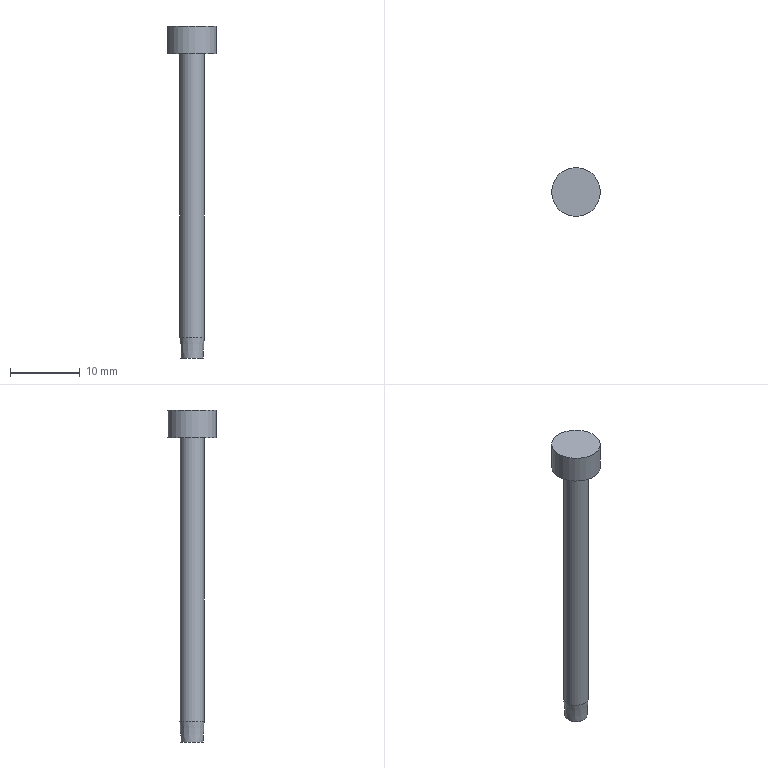Part | NX | features solid 2 | 1 solid | 6 faces | box 7 x 7 x 47.69 mm | volume 571.768 mm3 | plane 3 | cylinder 2 | cone 1 | commonest cylinder face diameters 3.5 x1 7 x1
STEP:
#1=CARTESIAN_POINT('',(-31.9,0.,66.5));
#2=VERTEX_POINT('',#1);
#3=CARTESIAN_POINT('',(-30.15,0.,66.5));
#4=DIRECTION('',(0.,0.,-1.));
#5=DIRECTION('',(-1.,0.,0.));
#6=AXIS2_PLACEMENT_3D('',#3,#4,#5);
#7=CIRCLE('',#6,1.75);
#8=EDGE_CURVE('',#2,#2,#7,.T.);
#9=ORIENTED_EDGE('',*,*,#8,.T.);
#10=EDGE_LOOP('',(#9));
#11=FACE_BOUND('',#10,.T.);
#12=CARTESIAN_POINT('',(-28.4,0.,25.81));
#13=VERTEX_POINT('',#12);
#14=CARTESIAN_POINT('',(-30.15,0.,25.81));
#15=DIRECTION('',(0.,0.,1.));
#16=DIRECTION('',(1.,0.,0.));
#17=AXIS2_PLACEMENT_3D('',#14,#15,#16);
#18=CIRCLE('',#17,1.75);
#19=EDGE_CURVE('',#13,#13,#18,.F.);
#20=ORIENTED_EDGE('',*,*,#19,.F.);
#21=EDGE_LOOP('',(#20));
#22=FACE_BOUND('',#21,.T.);
#23=CARTESIAN_POINT('',(-30.15,0.,-24.5));
#24=DIRECTION('',(0.,0.,1.));
#25=DIRECTION('',(1.,0.,0.));
#26=AXIS2_PLACEMENT_3D('',#23,#24,#25);
#27=CYLINDRICAL_SURFACE('',#26,1.75);
#28=ADVANCED_FACE('',(#11,#22),#27,.T.);
#29=CARTESIAN_POINT('',(-33.65,0.,66.5));
#30=VERTEX_POINT('',#29);
#31=CARTESIAN_POINT('',(-30.15,0.,66.5));
#32=DIRECTION('',(0.,0.,-1.));
#33=DIRECTION('',(-1.,0.,0.));
#34=AXIS2_PLACEMENT_3D('',#31,#32,#33);
#35=CIRCLE('',#34,3.5);
#36=EDGE_CURVE('',#30,#30,#35,.T.);
#37=ORIENTED_EDGE('',*,*,#36,.T.);
#38=EDGE_LOOP('',(#37));
#39=FACE_BOUND('',#38,.T.);
#40=ORIENTED_EDGE('',*,*,#8,.F.);
#41=EDGE_LOOP('',(#40));
#42=FACE_BOUND('',#41,.T.);
#43=CARTESIAN_POINT('',(-30.15,0.,66.5));
#44=DIRECTION('',(0.,0.,-1.));
#45=DIRECTION('',(-1.,0.,0.));
#46=AXIS2_PLACEMENT_3D('',#43,#44,#45);
#47=PLANE('',#46);
#48=ADVANCED_FACE('',(#39,#42),#47,.T.);
#49=ORIENTED_EDGE('',*,*,#36,.F.);
#50=EDGE_LOOP('',(#49));
#51=FACE_BOUND('',#50,.T.);
#52=CARTESIAN_POINT('',(-33.65,0.,70.5));
#53=VERTEX_POINT('',#52);
#54=CARTESIAN_POINT('',(-30.15,0.,70.5));
#55=DIRECTION('',(0.,0.,-1.));
#56=DIRECTION('',(-1.,0.,0.));
#57=AXIS2_PLACEMENT_3D('',#54,#55,#56);
#58=CIRCLE('',#57,3.5);
#59=EDGE_CURVE('',#53,#53,#58,.T.);
#60=ORIENTED_EDGE('',*,*,#59,.T.);
#61=EDGE_LOOP('',(#60));
#62=FACE_BOUND('',#61,.T.);
#63=CARTESIAN_POINT('',(-30.15,0.,66.5));
#64=DIRECTION('',(0.,0.,1.));
#65=DIRECTION('',(1.,0.,0.));
#66=AXIS2_PLACEMENT_3D('',#63,#64,#65);
#67=CYLINDRICAL_SURFACE('',#66,3.5);
#68=ADVANCED_FACE('',(#51,#62),#67,.T.);
#69=ORIENTED_EDGE('',*,*,#59,.F.);
#70=EDGE_LOOP('',(#69));
#71=FACE_BOUND('',#70,.T.);
#72=CARTESIAN_POINT('',(-30.15,0.,70.5));
#73=DIRECTION('',(0.,0.,-1.));
#74=DIRECTION('',(-1.,0.,0.));
#75=AXIS2_PLACEMENT_3D('',#72,#73,#74);
#76=PLANE('',#75);
#77=ADVANCED_FACE('',(#71),#76,.F.);
#78=CARTESIAN_POINT('',(-31.743,0.,22.81));
#79=VERTEX_POINT('',#78);
#80=CARTESIAN_POINT('',(-30.15,0.,22.81));
#81=DIRECTION('',(0.,0.,-1.));
#82=DIRECTION('',(-1.,0.,0.));
#83=AXIS2_PLACEMENT_3D('',#80,#81,#82);
#84=CIRCLE('',#83,1.593);
#85=EDGE_CURVE('',#79,#79,#84,.T.);
#86=ORIENTED_EDGE('',*,*,#85,.F.);
#87=EDGE_LOOP('',(#86));
#88=FACE_BOUND('',#87,.T.);
#89=ORIENTED_EDGE('',*,*,#19,.T.);
#90=EDGE_LOOP('',(#89));
#91=FACE_BOUND('',#90,.T.);
#92=CARTESIAN_POINT('',(-30.15,0.,25.81));
#93=DIRECTION('',(0.,0.,1.));
#94=DIRECTION('',(1.,0.,0.));
#95=AXIS2_PLACEMENT_3D('',#92,#93,#94);
#96=CONICAL_SURFACE('',#95,1.75,0.05236);
#97=ADVANCED_FACE('',(#88,#91),#96,.T.);
#98=ORIENTED_EDGE('',*,*,#85,.T.);
#99=EDGE_LOOP('',(#98));
#100=FACE_BOUND('',#99,.T.);
#101=CARTESIAN_POINT('',(-30.15,0.,22.81));
#102=DIRECTION('',(0.,0.,-1.));
#103=DIRECTION('',(-1.,0.,0.));
#104=AXIS2_PLACEMENT_3D('',#101,#102,#103);
#105=PLANE('',#104);
#106=ADVANCED_FACE('',(#100),#105,.T.);
#107=CLOSED_SHELL('',(#28,#48,#68,#77,#97,#106));
#108=MANIFOLD_SOLID_BREP('',#107);
#109=(LENGTH_UNIT()NAMED_UNIT(*)SI_UNIT(.MILLI.,.METRE.));
#110=UNCERTAINTY_MEASURE_WITH_UNIT(LENGTH_MEASURE(0.00001),#109,'','');
#111=(NAMED_UNIT(*)PLANE_ANGLE_UNIT()SI_UNIT($,.RADIAN.));
#112=(NAMED_UNIT(*)SI_UNIT($,.STERADIAN.)SOLID_ANGLE_UNIT());
#113=(GEOMETRIC_REPRESENTATION_CONTEXT(3)GLOBAL_UNCERTAINTY_ASSIGNED_CONTEXT((#110))GLOBAL_UNIT_ASSIGNED_CONTEXT((#109,#111,#112))REPRESENTATION_CONTEXT('',''));
#114=ADVANCED_BREP_SHAPE_REPRESENTATION('',(#108),#113);